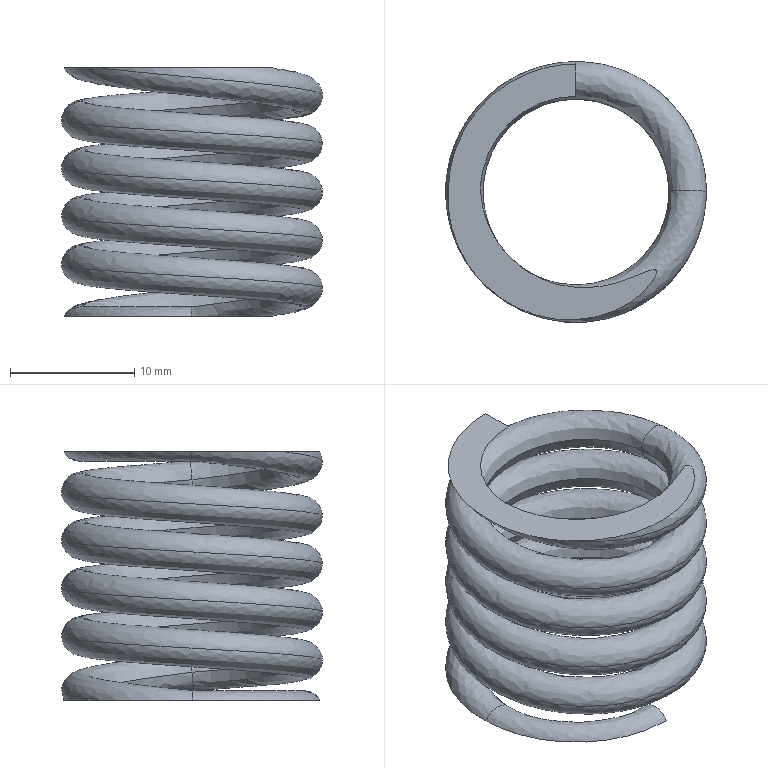Part | SolidWorks | features Helix 3, Cut 2, CompositeCurve 1, Sweep 1 | 1 solid | 12 faces | box 21 x 21 x 20 mm | volume 1917 mm3 | spline 8 | plane 4